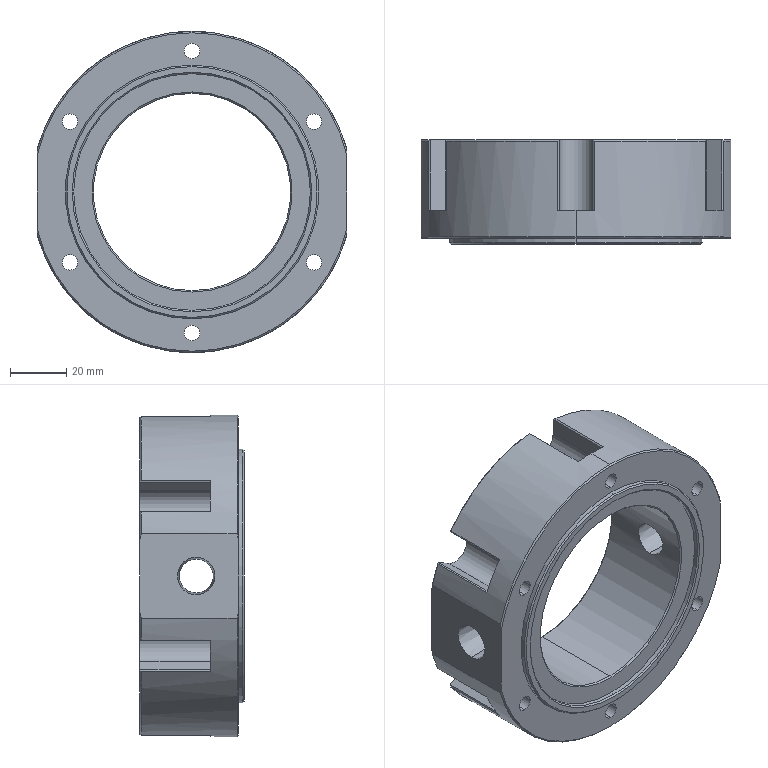Part | STEP file | 10-04 bearing seat cover plate upper | 1 solid | 89 faces | box 110 x 37 x 114 mm | volume 193708 mm3 | plane 36 | cylinder 30 | cone 23 | commonest cylinder face diameters 5.5 x12 12 x9 114 x3 70 x2 84 x2 90 x2